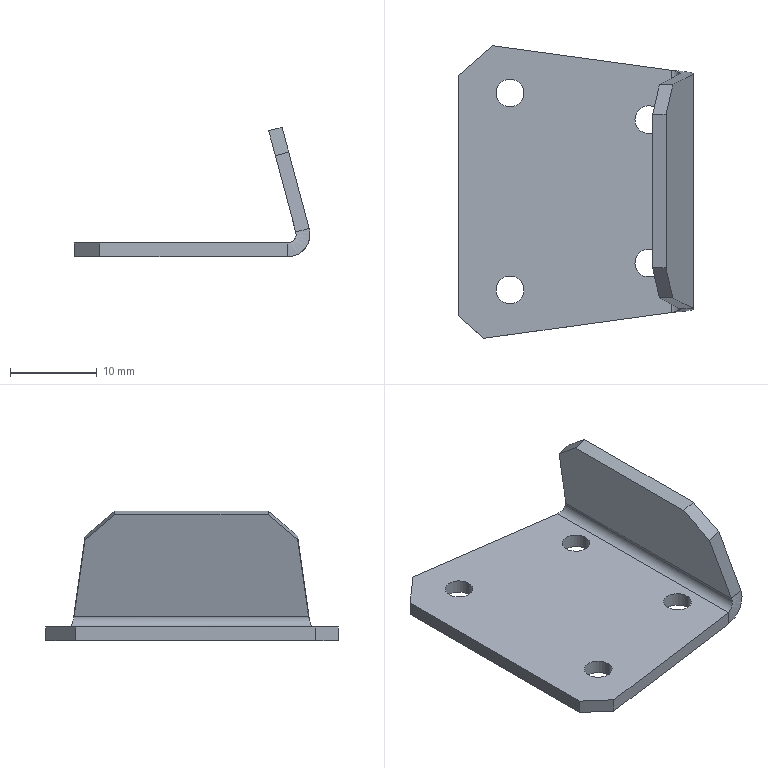Part | SolidWorks | features BaseBody 1 | 1 solid | 26 faces | box 27.212 x 33.746 x 14.951 mm | volume 1783 mm3 | plane 14 | cylinder 10 | spline 2 | commonest cylinder face diameters 3.2 x8 2 x1 5.2 x1
STEP:
#1=CARTESIAN_POINT('',(3.6,8.269,-1.6));
#2=VERTEX_POINT('',#1);
#3=CARTESIAN_POINT('',(0.4,8.269,-1.6));
#4=VERTEX_POINT('',#3);
#5=CARTESIAN_POINT('',(2.,8.269,-1.6));
#6=DIRECTION('',(0.,0.,-1.));
#7=DIRECTION('',(1.,0.,0.));
#8=AXIS2_PLACEMENT_3D('',#5,#6,#7);
#9=CIRCLE('',#8,1.6);
#10=EDGE_CURVE('',#2,#4,#9,.T.);
#11=ORIENTED_EDGE('',*,*,#10,.T.);
#12=CARTESIAN_POINT('',(0.4,8.269,0.));
#13=VERTEX_POINT('',#12);
#14=CARTESIAN_POINT('',(0.4,8.269,-1.6));
#15=DIRECTION('',(0.,0.,1.));
#16=VECTOR('',#15,1000.);
#17=LINE('',#14,#16);
#18=EDGE_CURVE('',#4,#13,#17,.T.);
#19=ORIENTED_EDGE('',*,*,#18,.T.);
#20=CARTESIAN_POINT('',(3.6,8.269,0.));
#21=VERTEX_POINT('',#20);
#22=CARTESIAN_POINT('',(2.,8.269,0.));
#23=DIRECTION('',(0.,0.,-1.));
#24=DIRECTION('',(1.,0.,0.));
#25=AXIS2_PLACEMENT_3D('',#22,#23,#24);
#26=CIRCLE('',#25,1.6);
#27=EDGE_CURVE('',#21,#13,#26,.T.);
#28=ORIENTED_EDGE('',*,*,#27,.F.);
#29=CARTESIAN_POINT('',(3.6,8.269,-1.6));
#30=DIRECTION('',(0.,0.,1.));
#31=VECTOR('',#30,1000.);
#32=LINE('',#29,#31);
#33=EDGE_CURVE('',#2,#21,#32,.T.);
#34=ORIENTED_EDGE('',*,*,#33,.F.);
#35=EDGE_LOOP('',(#11,#19,#28,#34));
#36=FACE_OUTER_BOUND('',#35,.T.);
#37=CARTESIAN_POINT('',(2.,8.269,-1.6));
#38=DIRECTION('',(0.,0.,1.));
#39=DIRECTION('',(1.,0.,0.));
#40=AXIS2_PLACEMENT_3D('',#37,#38,#39);
#41=CYLINDRICAL_SURFACE('',#40,1.6);
#42=ADVANCED_FACE('',(#36),#41,.F.);
#43=CARTESIAN_POINT('',(3.6,-8.269,-1.6));
#44=VERTEX_POINT('',#43);
#45=CARTESIAN_POINT('',(0.4,-8.269,-1.6));
#46=VERTEX_POINT('',#45);
#47=CARTESIAN_POINT('',(2.,-8.269,-1.6));
#48=DIRECTION('',(0.,0.,-1.));
#49=DIRECTION('',(1.,0.,0.));
#50=AXIS2_PLACEMENT_3D('',#47,#48,#49);
#51=CIRCLE('',#50,1.6);
#52=EDGE_CURVE('',#44,#46,#51,.T.);
#53=ORIENTED_EDGE('',*,*,#52,.T.);
#54=CARTESIAN_POINT('',(0.4,-8.269,0.));
#55=VERTEX_POINT('',#54);
#56=CARTESIAN_POINT('',(0.4,-8.269,-1.6));
#57=DIRECTION('',(0.,0.,1.));
#58=VECTOR('',#57,1000.);
#59=LINE('',#56,#58);
#60=EDGE_CURVE('',#46,#55,#59,.T.);
#61=ORIENTED_EDGE('',*,*,#60,.T.);
#62=CARTESIAN_POINT('',(3.6,-8.269,0.));
#63=VERTEX_POINT('',#62);
#64=CARTESIAN_POINT('',(2.,-8.269,0.));
#65=DIRECTION('',(0.,0.,-1.));
#66=DIRECTION('',(1.,0.,0.));
#67=AXIS2_PLACEMENT_3D('',#64,#65,#66);
#68=CIRCLE('',#67,1.6);
#69=EDGE_CURVE('',#63,#55,#68,.T.);
#70=ORIENTED_EDGE('',*,*,#69,.F.);
#71=CARTESIAN_POINT('',(3.6,-8.269,-1.6));
#72=DIRECTION('',(0.,0.,1.));
#73=VECTOR('',#72,1000.);
#74=LINE('',#71,#73);
#75=EDGE_CURVE('',#44,#63,#74,.T.);
#76=ORIENTED_EDGE('',*,*,#75,.F.);
#77=EDGE_LOOP('',(#53,#61,#70,#76));
#78=FACE_OUTER_BOUND('',#77,.T.);
#79=CARTESIAN_POINT('',(2.,-8.269,-1.6));
#80=DIRECTION('',(0.,0.,1.));
#81=DIRECTION('',(1.,0.,0.));
#82=AXIS2_PLACEMENT_3D('',#79,#80,#81);
#83=CYLINDRICAL_SURFACE('',#82,1.6);
#84=ADVANCED_FACE('',(#78),#83,.F.);
#85=CARTESIAN_POINT('',(-12.4,-11.35,-1.6));
#86=VERTEX_POINT('',#85);
#87=CARTESIAN_POINT('',(-15.6,-11.35,-1.6));
#88=VERTEX_POINT('',#87);
#89=CARTESIAN_POINT('',(-14.,-11.35,-1.6));
#90=DIRECTION('',(0.,0.,-1.));
#91=DIRECTION('',(1.,0.,0.));
#92=AXIS2_PLACEMENT_3D('',#89,#90,#91);
#93=CIRCLE('',#92,1.6);
#94=EDGE_CURVE('',#86,#88,#93,.T.);
#95=ORIENTED_EDGE('',*,*,#94,.T.);
#96=CARTESIAN_POINT('',(-15.6,-11.35,0.));
#97=VERTEX_POINT('',#96);
#98=CARTESIAN_POINT('',(-15.6,-11.35,-1.6));
#99=DIRECTION('',(0.,0.,1.));
#100=VECTOR('',#99,1000.);
#101=LINE('',#98,#100);
#102=EDGE_CURVE('',#88,#97,#101,.T.);
#103=ORIENTED_EDGE('',*,*,#102,.T.);
#104=CARTESIAN_POINT('',(-12.4,-11.35,0.));
#105=VERTEX_POINT('',#104);
#106=CARTESIAN_POINT('',(-14.,-11.35,0.));
#107=DIRECTION('',(0.,0.,-1.));
#108=DIRECTION('',(1.,0.,0.));
#109=AXIS2_PLACEMENT_3D('',#106,#107,#108);
#110=CIRCLE('',#109,1.6);
#111=EDGE_CURVE('',#105,#97,#110,.T.);
#112=ORIENTED_EDGE('',*,*,#111,.F.);
#113=CARTESIAN_POINT('',(-12.4,-11.35,-1.6));
#114=DIRECTION('',(0.,0.,1.));
#115=VECTOR('',#114,1000.);
#116=LINE('',#113,#115);
#117=EDGE_CURVE('',#86,#105,#116,.T.);
#118=ORIENTED_EDGE('',*,*,#117,.F.);
#119=EDGE_LOOP('',(#95,#103,#112,#118));
#120=FACE_OUTER_BOUND('',#119,.T.);
#121=CARTESIAN_POINT('',(-14.,-11.35,-1.6));
#122=DIRECTION('',(0.,0.,1.));
#123=DIRECTION('',(1.,0.,0.));
#124=AXIS2_PLACEMENT_3D('',#121,#122,#123);
#125=CYLINDRICAL_SURFACE('',#124,1.6);
#126=ADVANCED_FACE('',(#120),#125,.F.);
#127=CARTESIAN_POINT('',(-12.4,11.35,-1.6));
#128=VERTEX_POINT('',#127);
#129=CARTESIAN_POINT('',(-15.6,11.35,-1.6));
#130=VERTEX_POINT('',#129);
#131=CARTESIAN_POINT('',(-14.,11.35,-1.6));
#132=DIRECTION('',(0.,0.,-1.));
#133=DIRECTION('',(1.,0.,0.));
#134=AXIS2_PLACEMENT_3D('',#131,#132,#133);
#135=CIRCLE('',#134,1.6);
#136=EDGE_CURVE('',#128,#130,#135,.T.);
#137=ORIENTED_EDGE('',*,*,#136,.T.);
#138=CARTESIAN_POINT('',(-15.6,11.35,0.));
#139=VERTEX_POINT('',#138);
#140=CARTESIAN_POINT('',(-15.6,11.35,-1.6));
#141=DIRECTION('',(0.,0.,1.));
#142=VECTOR('',#141,1000.);
#143=LINE('',#140,#142);
#144=EDGE_CURVE('',#130,#139,#143,.T.);
#145=ORIENTED_EDGE('',*,*,#144,.T.);
#146=CARTESIAN_POINT('',(-12.4,11.35,0.));
#147=VERTEX_POINT('',#146);
#148=CARTESIAN_POINT('',(-14.,11.35,0.));
#149=DIRECTION('',(0.,0.,-1.));
#150=DIRECTION('',(1.,0.,0.));
#151=AXIS2_PLACEMENT_3D('',#148,#149,#150);
#152=CIRCLE('',#151,1.6);
#153=EDGE_CURVE('',#147,#139,#152,.T.);
#154=ORIENTED_EDGE('',*,*,#153,.F.);
#155=CARTESIAN_POINT('',(-12.4,11.35,-1.6));
#156=DIRECTION('',(0.,0.,1.));
#157=VECTOR('',#156,1000.);
#158=LINE('',#155,#157);
#159=EDGE_CURVE('',#128,#147,#158,.T.);
#160=ORIENTED_EDGE('',*,*,#159,.F.);
#161=EDGE_LOOP('',(#137,#145,#154,#160));
#162=FACE_OUTER_BOUND('',#161,.T.);
#163=CARTESIAN_POINT('',(-14.,11.35,-1.6));
#164=DIRECTION('',(0.,0.,1.));
#165=DIRECTION('',(1.,0.,0.));
#166=AXIS2_PLACEMENT_3D('',#163,#164,#165);
#167=CYLINDRICAL_SURFACE('',#166,1.6);
#168=ADVANCED_FACE('',(#162),#167,.F.);
#169=CARTESIAN_POINT('',(5.578,-13.512,1.259));
#170=VERTEX_POINT('',#169);
#171=CARTESIAN_POINT('',(4.612,-13.966,0.));
#172=VERTEX_POINT('',#171);
#173=CARTESIAN_POINT('',(5.578,-13.512,1.259));
#174=CARTESIAN_POINT('',(5.617,-13.55,1.11));
#175=CARTESIAN_POINT('',(5.622,-13.588,0.9534));
#176=CARTESIAN_POINT('',(5.563,-13.663,0.6556));
#177=CARTESIAN_POINT('',(5.498,-13.701,0.513));
#178=CARTESIAN_POINT('',(5.312,-13.777,0.2701));
#179=CARTESIAN_POINT('',(5.191,-13.815,0.1708));
#180=CARTESIAN_POINT('',(4.917,-13.89,0.03575));
#181=CARTESIAN_POINT('',(4.766,-13.928,0.));
#182=CARTESIAN_POINT('',(4.612,-13.966,0.));
#183=B_SPLINE_CURVE_WITH_KNOTS('',3,(#173,#174,#175,#176,#177,#178,#179,#180,#181,#182),.UNSPECIFIED.,.F.,.F.,(4,2,2,2,4),(-0.0002673,0.0002018,0.000671,0.00114,0.001609),.UNSPECIFIED.);
#184=EDGE_CURVE('',#170,#172,#183,.T.);
#185=ORIENTED_EDGE('',*,*,#184,.F.);
#186=CARTESIAN_POINT('',(5.578,13.512,1.259));
#187=VERTEX_POINT('',#186);
#188=CARTESIAN_POINT('',(5.578,0.,1.259));
#189=DIRECTION('',(0.,1.,0.));
#190=VECTOR('',#189,1000.);
#191=LINE('',#188,#190);
#192=EDGE_CURVE('',#170,#187,#191,.T.);
#193=ORIENTED_EDGE('',*,*,#192,.T.);
#194=CARTESIAN_POINT('',(4.612,13.966,0.));
#195=VERTEX_POINT('',#194);
#196=CARTESIAN_POINT('',(4.612,13.966,0.));
#197=CARTESIAN_POINT('',(4.689,13.947,0.));
#198=CARTESIAN_POINT('',(4.764,13.928,0.008783));
#199=CARTESIAN_POINT('',(4.912,13.891,0.04322));
#200=CARTESIAN_POINT('',(4.985,13.871,0.06937));
#201=CARTESIAN_POINT('',(5.19,13.815,0.1702));
#202=CARTESIAN_POINT('',(5.311,13.777,0.2697));
#203=CARTESIAN_POINT('',(5.45,13.721,0.4504));
#204=CARTESIAN_POINT('',(5.491,13.702,0.517));
#205=CARTESIAN_POINT('',(5.553,13.664,0.6555));
#206=CARTESIAN_POINT('',(5.577,13.645,0.7278));
#207=CARTESIAN_POINT('',(5.622,13.588,0.9536));
#208=CARTESIAN_POINT('',(5.617,13.55,1.11));
#209=CARTESIAN_POINT('',(5.578,13.512,1.259));
#210=B_SPLINE_CURVE_WITH_KNOTS('',3,(#196,#197,#198,#199,#200,#201,#202,#203,#204,#205,#206,#207,#208,#209),.UNSPECIFIED.,.F.,.F.,(4,2,2,2,2,2,4),(-0.001619,-0.001383,-0.001147,-0.0006751,-0.0004391,-0.0002031,0.000269),.UNSPECIFIED.);
#211=EDGE_CURVE('',#195,#187,#210,.T.);
#212=ORIENTED_EDGE('',*,*,#211,.F.);
#213=CARTESIAN_POINT('',(4.612,0.,0.));
#214=DIRECTION('',(0.,-1.,0.));
#215=VECTOR('',#214,1000.);
#216=LINE('',#213,#215);
#217=EDGE_CURVE('',#195,#172,#216,.T.);
#218=ORIENTED_EDGE('',*,*,#217,.T.);
#219=EDGE_LOOP('',(#185,#193,#212,#218));
#220=FACE_OUTER_BOUND('',#219,.T.);
#221=CARTESIAN_POINT('',(4.612,13.74,1.));
#222=DIRECTION('',(0.,-1.,0.));
#223=DIRECTION('',(0.,0.,-1.));
#224=AXIS2_PLACEMENT_3D('',#221,#222,#223);
#225=CYLINDRICAL_SURFACE('',#224,1.);
#226=ADVANCED_FACE('',(#220),#225,.F.);
#227=CARTESIAN_POINT('',(2.448,8.85,12.937));
#228=VERTEX_POINT('',#227);
#229=CARTESIAN_POINT('',(3.218,12.259,10.066));
#230=VERTEX_POINT('',#229);
#231=CARTESIAN_POINT('',(2.448,8.85,12.937));
#232=DIRECTION('',(0.1701,0.7537,-0.6348));
#233=VECTOR('',#232,1000.);
#234=LINE('',#231,#233);
#235=EDGE_CURVE('',#228,#230,#234,.T.);
#236=ORIENTED_EDGE('',*,*,#235,.T.);
#237=CARTESIAN_POINT('',(3.218,12.259,10.066));
#238=DIRECTION('',(0.2564,0.1362,-0.9569));
#239=VECTOR('',#238,1000.);
#240=LINE('',#237,#239);
#241=EDGE_CURVE('',#230,#187,#240,.T.);
#242=ORIENTED_EDGE('',*,*,#241,.T.);
#243=ORIENTED_EDGE('',*,*,#192,.F.);
#244=CARTESIAN_POINT('',(3.218,-12.259,10.066));
#245=VERTEX_POINT('',#244);
#246=CARTESIAN_POINT('',(5.578,-13.512,1.259));
#247=DIRECTION('',(-0.2564,0.1362,0.9569));
#248=VECTOR('',#247,1000.);
#249=LINE('',#246,#248);
#250=EDGE_CURVE('',#170,#245,#249,.T.);
#251=ORIENTED_EDGE('',*,*,#250,.T.);
#252=CARTESIAN_POINT('',(2.448,-8.85,12.937));
#253=VERTEX_POINT('',#252);
#254=CARTESIAN_POINT('',(3.218,-12.259,10.066));
#255=DIRECTION('',(-0.1701,0.7537,0.6348));
#256=VECTOR('',#255,1000.);
#257=LINE('',#254,#256);
#258=EDGE_CURVE('',#245,#253,#257,.T.);
#259=ORIENTED_EDGE('',*,*,#258,.T.);
#260=CARTESIAN_POINT('',(2.448,0.,12.937));
#261=DIRECTION('',(0.,1.,0.));
#262=VECTOR('',#261,1000.);
#263=LINE('',#260,#262);
#264=EDGE_CURVE('',#253,#228,#263,.T.);
#265=ORIENTED_EDGE('',*,*,#264,.T.);
#266=EDGE_LOOP('',(#236,#242,#243,#251,#259,#265));
#267=FACE_OUTER_BOUND('',#266,.T.);
#268=CARTESIAN_POINT('',(5.578,-13.512,1.259));
#269=DIRECTION('',(-0.9659,0.,-0.2588));
#270=DIRECTION('',(-0.2588,0.,0.9659));
#271=AXIS2_PLACEMENT_3D('',#268,#269,#270);
#272=PLANE('',#271);
#273=ADVANCED_FACE('',(#267),#272,.T.);
#274=CARTESIAN_POINT('',(4.763,12.259,10.48));
#275=VERTEX_POINT('',#274);
#276=CARTESIAN_POINT('',(3.99,12.259,10.273));
#277=DIRECTION('',(0.9659,0.,0.2588));
#278=VECTOR('',#277,1000.);
#279=LINE('',#276,#278);
#280=EDGE_CURVE('',#230,#275,#279,.T.);
#281=ORIENTED_EDGE('',*,*,#280,.T.);
#282=CARTESIAN_POINT('',(7.123,13.512,1.673));
#283=VERTEX_POINT('',#282);
#284=CARTESIAN_POINT('',(5.943,12.885,6.076));
#285=DIRECTION('',(0.2564,0.1362,-0.9569));
#286=VECTOR('',#285,1000.);
#287=LINE('',#284,#286);
#288=EDGE_CURVE('',#275,#283,#287,.T.);
#289=ORIENTED_EDGE('',*,*,#288,.T.);
#290=CARTESIAN_POINT('',(6.35,13.512,1.466));
#291=DIRECTION('',(0.9659,0.,0.2588));
#292=VECTOR('',#291,1000.);
#293=LINE('',#290,#292);
#294=EDGE_CURVE('',#187,#283,#293,.T.);
#295=ORIENTED_EDGE('',*,*,#294,.F.);
#296=ORIENTED_EDGE('',*,*,#241,.F.);
#297=EDGE_LOOP('',(#281,#289,#295,#296));
#298=FACE_OUTER_BOUND('',#297,.T.);
#299=CARTESIAN_POINT('',(4.763,12.259,10.48));
#300=DIRECTION('',(-0.03526,0.9907,0.1316));
#301=DIRECTION('',(0.2564,0.1362,-0.9569));
#302=AXIS2_PLACEMENT_3D('',#299,#300,#301);
#303=PLANE('',#302);
#304=ADVANCED_FACE('',(#298),#303,.T.);
#305=CARTESIAN_POINT('',(3.994,8.85,13.351));
#306=VERTEX_POINT('',#305);
#307=CARTESIAN_POINT('',(4.379,10.554,11.915));
#308=DIRECTION('',(0.1701,0.7537,-0.6348));
#309=VECTOR('',#308,1000.);
#310=LINE('',#307,#309);
#311=EDGE_CURVE('',#306,#275,#310,.T.);
#312=ORIENTED_EDGE('',*,*,#311,.T.);
#313=ORIENTED_EDGE('',*,*,#280,.F.);
#314=ORIENTED_EDGE('',*,*,#235,.F.);
#315=CARTESIAN_POINT('',(3.221,8.85,13.144));
#316=DIRECTION('',(0.9659,0.,0.2588));
#317=VECTOR('',#316,1000.);
#318=LINE('',#315,#317);
#319=EDGE_CURVE('',#228,#306,#318,.T.);
#320=ORIENTED_EDGE('',*,*,#319,.T.);
#321=EDGE_LOOP('',(#312,#313,#314,#320));
#322=FACE_OUTER_BOUND('',#321,.T.);
#323=CARTESIAN_POINT('',(3.994,8.85,13.351));
#324=DIRECTION('',(-0.1951,0.6572,0.728));
#325=DIRECTION('',(0.1701,0.7537,-0.6348));
#326=AXIS2_PLACEMENT_3D('',#323,#324,#325);
#327=PLANE('',#326);
#328=ADVANCED_FACE('',(#322),#327,.T.);
#329=CARTESIAN_POINT('',(3.994,-8.85,13.351));
#330=VERTEX_POINT('',#329);
#331=CARTESIAN_POINT('',(3.994,0.,13.351));
#332=DIRECTION('',(0.,1.,0.));
#333=VECTOR('',#332,1000.);
#334=LINE('',#331,#333);
#335=EDGE_CURVE('',#330,#306,#334,.T.);
#336=ORIENTED_EDGE('',*,*,#335,.T.);
#337=ORIENTED_EDGE('',*,*,#319,.F.);
#338=ORIENTED_EDGE('',*,*,#264,.F.);
#339=CARTESIAN_POINT('',(3.221,-8.85,13.144));
#340=DIRECTION('',(0.9659,0.,0.2588));
#341=VECTOR('',#340,1000.);
#342=LINE('',#339,#341);
#343=EDGE_CURVE('',#253,#330,#342,.T.);
#344=ORIENTED_EDGE('',*,*,#343,.T.);
#345=EDGE_LOOP('',(#336,#337,#338,#344));
#346=FACE_OUTER_BOUND('',#345,.T.);
#347=CARTESIAN_POINT('',(2.448,-8.85,12.937));
#348=DIRECTION('',(-0.2588,0.,0.9659));
#349=DIRECTION('',(0.9659,0.,0.2588));
#350=AXIS2_PLACEMENT_3D('',#347,#348,#349);
#351=PLANE('',#350);
#352=ADVANCED_FACE('',(#346),#351,.T.);
#353=CARTESIAN_POINT('',(4.763,-12.259,10.48));
#354=VERTEX_POINT('',#353);
#355=CARTESIAN_POINT('',(4.379,-10.554,11.915));
#356=DIRECTION('',(-0.1701,0.7537,0.6348));
#357=VECTOR('',#356,1000.);
#358=LINE('',#355,#357);
#359=EDGE_CURVE('',#354,#330,#358,.T.);
#360=ORIENTED_EDGE('',*,*,#359,.T.);
#361=ORIENTED_EDGE('',*,*,#343,.F.);
#362=ORIENTED_EDGE('',*,*,#258,.F.);
#363=CARTESIAN_POINT('',(3.99,-12.259,10.273));
#364=DIRECTION('',(0.9659,0.,0.2588));
#365=VECTOR('',#364,1000.);
#366=LINE('',#363,#365);
#367=EDGE_CURVE('',#245,#354,#366,.T.);
#368=ORIENTED_EDGE('',*,*,#367,.T.);
#369=EDGE_LOOP('',(#360,#361,#362,#368));
#370=FACE_OUTER_BOUND('',#369,.T.);
#371=CARTESIAN_POINT('',(4.763,-12.259,10.48));
#372=DIRECTION('',(-0.1951,-0.6572,0.728));
#373=DIRECTION('',(-0.1701,0.7537,0.6348));
#374=AXIS2_PLACEMENT_3D('',#371,#372,#373);
#375=PLANE('',#374);
#376=ADVANCED_FACE('',(#370),#375,.T.);
#377=ORIENTED_EDGE('',*,*,#367,.F.);
#378=ORIENTED_EDGE('',*,*,#250,.F.);
#379=CARTESIAN_POINT('',(7.123,-13.512,1.673));
#380=VERTEX_POINT('',#379);
#381=CARTESIAN_POINT('',(6.35,-13.512,1.466));
#382=DIRECTION('',(-0.9659,0.,-0.2588));
#383=VECTOR('',#382,1000.);
#384=LINE('',#381,#383);
#385=EDGE_CURVE('',#380,#170,#384,.T.);
#386=ORIENTED_EDGE('',*,*,#385,.F.);
#387=CARTESIAN_POINT('',(5.943,-12.885,6.076));
#388=DIRECTION('',(-0.2564,0.1362,0.9569));
#389=VECTOR('',#388,1000.);
#390=LINE('',#387,#389);
#391=EDGE_CURVE('',#380,#354,#390,.T.);
#392=ORIENTED_EDGE('',*,*,#391,.T.);
#393=EDGE_LOOP('',(#377,#378,#386,#392));
#394=FACE_OUTER_BOUND('',#393,.T.);
#395=CARTESIAN_POINT('',(7.123,-13.512,1.673));
#396=DIRECTION('',(-0.03526,-0.9907,0.1316));
#397=DIRECTION('',(-0.2564,0.1362,0.9569));
#398=AXIS2_PLACEMENT_3D('',#395,#396,#397);
#399=PLANE('',#398);
#400=ADVANCED_FACE('',(#394),#399,.T.);
#401=ORIENTED_EDGE('',*,*,#27,.T.);
#402=CARTESIAN_POINT('',(2.,8.269,0.));
#403=DIRECTION('',(0.,0.,-1.));
#404=DIRECTION('',(1.,0.,0.));
#405=AXIS2_PLACEMENT_3D('',#402,#403,#404);
#406=CIRCLE('',#405,1.6);
#407=EDGE_CURVE('',#13,#21,#406,.T.);
#408=ORIENTED_EDGE('',*,*,#407,.T.);
#409=EDGE_LOOP('',(#401,#408));
#410=FACE_BOUND('',#409,.T.);
#411=ORIENTED_EDGE('',*,*,#69,.T.);
#412=CARTESIAN_POINT('',(2.,-8.269,0.));
#413=DIRECTION('',(0.,0.,-1.));
#414=DIRECTION('',(1.,0.,0.));
#415=AXIS2_PLACEMENT_3D('',#412,#413,#414);
#416=CIRCLE('',#415,1.6);
#417=EDGE_CURVE('',#55,#63,#416,.T.);
#418=ORIENTED_EDGE('',*,*,#417,.T.);
#419=EDGE_LOOP('',(#411,#418));
#420=FACE_BOUND('',#419,.T.);
#421=ORIENTED_EDGE('',*,*,#111,.T.);
#422=CARTESIAN_POINT('',(-14.,-11.35,0.));
#423=DIRECTION('',(0.,0.,-1.));
#424=DIRECTION('',(1.,0.,0.));
#425=AXIS2_PLACEMENT_3D('',#422,#423,#424);
#426=CIRCLE('',#425,1.6);
#427=EDGE_CURVE('',#97,#105,#426,.T.);
#428=ORIENTED_EDGE('',*,*,#427,.T.);
#429=EDGE_LOOP('',(#421,#428));
#430=FACE_BOUND('',#429,.T.);
#431=ORIENTED_EDGE('',*,*,#153,.T.);
#432=CARTESIAN_POINT('',(-14.,11.35,0.));
#433=DIRECTION('',(0.,0.,-1.));
#434=DIRECTION('',(1.,0.,0.));
#435=AXIS2_PLACEMENT_3D('',#432,#433,#434);
#436=CIRCLE('',#435,1.6);
#437=EDGE_CURVE('',#139,#147,#436,.T.);
#438=ORIENTED_EDGE('',*,*,#437,.T.);
#439=EDGE_LOOP('',(#431,#438));
#440=FACE_BOUND('',#439,.T.);
#441=CARTESIAN_POINT('',(-20.,13.35,0.));
#442=VERTEX_POINT('',#441);
#443=CARTESIAN_POINT('',(-20.,-14.35,0.));
#444=VERTEX_POINT('',#443);
#445=CARTESIAN_POINT('',(-20.,-0.06811,0.));
#446=DIRECTION('',(0.,-1.,0.));
#447=VECTOR('',#446,1000.);
#448=LINE('',#445,#447);
#449=EDGE_CURVE('',#442,#444,#448,.T.);
#450=ORIENTED_EDGE('',*,*,#449,.T.);
#451=CARTESIAN_POINT('',(-17.028,-16.941,0.));
#452=VERTEX_POINT('',#451);
#453=CARTESIAN_POINT('',(-20.,-14.35,0.));
#454=DIRECTION('',(0.7537,-0.6572,0.));
#455=VECTOR('',#454,1000.);
#456=LINE('',#453,#455);
#457=EDGE_CURVE('',#444,#452,#456,.T.);
#458=ORIENTED_EDGE('',*,*,#457,.T.);
#459=CARTESIAN_POINT('',(-17.028,-16.941,0.));
#460=DIRECTION('',(0.9907,0.1362,0.));
#461=VECTOR('',#460,1000.);
#462=LINE('',#459,#461);
#463=EDGE_CURVE('',#452,#172,#462,.T.);
#464=ORIENTED_EDGE('',*,*,#463,.T.);
#465=ORIENTED_EDGE('',*,*,#217,.F.);
#466=CARTESIAN_POINT('',(-16.037,16.805,0.));
#467=VERTEX_POINT('',#466);
#468=CARTESIAN_POINT('',(4.612,13.966,0.));
#469=DIRECTION('',(-0.9907,0.1362,0.));
#470=VECTOR('',#469,1000.);
#471=LINE('',#468,#470);
#472=EDGE_CURVE('',#195,#467,#471,.T.);
#473=ORIENTED_EDGE('',*,*,#472,.T.);
#474=CARTESIAN_POINT('',(-16.037,16.805,0.));
#475=DIRECTION('',(-0.7537,-0.6572,0.));
#476=VECTOR('',#475,1000.);
#477=LINE('',#474,#476);
#478=EDGE_CURVE('',#467,#442,#477,.T.);
#479=ORIENTED_EDGE('',*,*,#478,.T.);
#480=EDGE_LOOP('',(#450,#458,#464,#465,#473,#479));
#481=FACE_OUTER_BOUND('',#480,.T.);
#482=CARTESIAN_POINT('',(-20.,-17.144,0.));
#483=DIRECTION('',(0.,0.,1.));
#484=DIRECTION('',(1.,0.,0.));
#485=AXIS2_PLACEMENT_3D('',#482,#483,#484);
#486=PLANE('',#485);
#487=ADVANCED_FACE('',(#410,#420,#430,#440,#481),#486,.T.);
#488=CARTESIAN_POINT('',(7.123,0.,1.673));
#489=DIRECTION('',(0.,-1.,0.));
#490=VECTOR('',#489,1000.);
#491=LINE('',#488,#490);
#492=EDGE_CURVE('',#283,#380,#491,.T.);
#493=ORIENTED_EDGE('',*,*,#492,.F.);
#494=ORIENTED_EDGE('',*,*,#288,.F.);
#495=ORIENTED_EDGE('',*,*,#311,.F.);
#496=ORIENTED_EDGE('',*,*,#335,.F.);
#497=ORIENTED_EDGE('',*,*,#359,.F.);
#498=ORIENTED_EDGE('',*,*,#391,.F.);
#499=EDGE_LOOP('',(#493,#494,#495,#496,#497,#498));
#500=FACE_OUTER_BOUND('',#499,.T.);
#501=CARTESIAN_POINT('',(7.123,-13.512,1.673));
#502=DIRECTION('',(-0.9659,0.,-0.2588));
#503=DIRECTION('',(-0.2588,0.,0.9659));
#504=AXIS2_PLACEMENT_3D('',#501,#502,#503);
#505=PLANE('',#504);
#506=ADVANCED_FACE('',(#500),#505,.F.);
#507=ORIENTED_EDGE('',*,*,#18,.F.);
#508=CARTESIAN_POINT('',(2.,8.269,-1.6));
#509=DIRECTION('',(0.,0.,-1.));
#510=DIRECTION('',(1.,0.,0.));
#511=AXIS2_PLACEMENT_3D('',#508,#509,#510);
#512=CIRCLE('',#511,1.6);
#513=EDGE_CURVE('',#4,#2,#512,.T.);
#514=ORIENTED_EDGE('',*,*,#513,.T.);
#515=ORIENTED_EDGE('',*,*,#33,.T.);
#516=ORIENTED_EDGE('',*,*,#407,.F.);
#517=EDGE_LOOP('',(#507,#514,#515,#516));
#518=FACE_OUTER_BOUND('',#517,.T.);
#519=CARTESIAN_POINT('',(2.,8.269,-1.6));
#520=DIRECTION('',(0.,0.,1.));
#521=DIRECTION('',(1.,0.,0.));
#522=AXIS2_PLACEMENT_3D('',#519,#520,#521);
#523=CYLINDRICAL_SURFACE('',#522,1.6);
#524=ADVANCED_FACE('',(#518),#523,.F.);
#525=ORIENTED_EDGE('',*,*,#60,.F.);
#526=CARTESIAN_POINT('',(2.,-8.269,-1.6));
#527=DIRECTION('',(0.,0.,-1.));
#528=DIRECTION('',(1.,0.,0.));
#529=AXIS2_PLACEMENT_3D('',#526,#527,#528);
#530=CIRCLE('',#529,1.6);
#531=EDGE_CURVE('',#46,#44,#530,.T.);
#532=ORIENTED_EDGE('',*,*,#531,.T.);
#533=ORIENTED_EDGE('',*,*,#75,.T.);
#534=ORIENTED_EDGE('',*,*,#417,.F.);
#535=EDGE_LOOP('',(#525,#532,#533,#534));
#536=FACE_OUTER_BOUND('',#535,.T.);
#537=CARTESIAN_POINT('',(2.,-8.269,-1.6));
#538=DIRECTION('',(0.,0.,1.));
#539=DIRECTION('',(1.,0.,0.));
#540=AXIS2_PLACEMENT_3D('',#537,#538,#539);
#541=CYLINDRICAL_SURFACE('',#540,1.6);
#542=ADVANCED_FACE('',(#536),#541,.F.);
#543=ORIENTED_EDGE('',*,*,#102,.F.);
#544=CARTESIAN_POINT('',(-14.,-11.35,-1.6));
#545=DIRECTION('',(0.,0.,-1.));
#546=DIRECTION('',(1.,0.,0.));
#547=AXIS2_PLACEMENT_3D('',#544,#545,#546);
#548=CIRCLE('',#547,1.6);
#549=EDGE_CURVE('',#88,#86,#548,.T.);
#550=ORIENTED_EDGE('',*,*,#549,.T.);
#551=ORIENTED_EDGE('',*,*,#117,.T.);
#552=ORIENTED_EDGE('',*,*,#427,.F.);
#553=EDGE_LOOP('',(#543,#550,#551,#552));
#554=FACE_OUTER_BOUND('',#553,.T.);
#555=CARTESIAN_POINT('',(-14.,-11.35,-1.6));
#556=DIRECTION('',(0.,0.,1.));
#557=DIRECTION('',(1.,0.,0.));
#558=AXIS2_PLACEMENT_3D('',#555,#556,#557);
#559=CYLINDRICAL_SURFACE('',#558,1.6);
#560=ADVANCED_FACE('',(#554),#559,.F.);
#561=ORIENTED_EDGE('',*,*,#144,.F.);
#562=CARTESIAN_POINT('',(-14.,11.35,-1.6));
#563=DIRECTION('',(0.,0.,-1.));
#564=DIRECTION('',(1.,0.,0.));
#565=AXIS2_PLACEMENT_3D('',#562,#563,#564);
#566=CIRCLE('',#565,1.6);
#567=EDGE_CURVE('',#130,#128,#566,.T.);
#568=ORIENTED_EDGE('',*,*,#567,.T.);
#569=ORIENTED_EDGE('',*,*,#159,.T.);
#570=ORIENTED_EDGE('',*,*,#437,.F.);
#571=EDGE_LOOP('',(#561,#568,#569,#570));
#572=FACE_OUTER_BOUND('',#571,.T.);
#573=CARTESIAN_POINT('',(-14.,11.35,-1.6));
#574=DIRECTION('',(0.,0.,1.));
#575=DIRECTION('',(1.,0.,0.));
#576=AXIS2_PLACEMENT_3D('',#573,#574,#575);
#577=CYLINDRICAL_SURFACE('',#576,1.6);
#578=ADVANCED_FACE('',(#572),#577,.F.);
#579=CARTESIAN_POINT('',(-20.,-14.35,-1.6));
#580=VERTEX_POINT('',#579);
#581=CARTESIAN_POINT('',(-17.028,-16.941,-1.6));
#582=VERTEX_POINT('',#581);
#583=CARTESIAN_POINT('',(-18.514,-15.646,-1.6));
#584=DIRECTION('',(0.7537,-0.6572,0.));
#585=VECTOR('',#584,1000.);
#586=LINE('',#583,#585);
#587=EDGE_CURVE('',#580,#582,#586,.T.);
#588=ORIENTED_EDGE('',*,*,#587,.T.);
#589=CARTESIAN_POINT('',(-17.028,-16.941,-0.8));
#590=DIRECTION('',(0.,0.,1.));
#591=VECTOR('',#590,1000.);
#592=LINE('',#589,#591);
#593=EDGE_CURVE('',#582,#452,#592,.T.);
#594=ORIENTED_EDGE('',*,*,#593,.T.);
#595=ORIENTED_EDGE('',*,*,#457,.F.);
#596=CARTESIAN_POINT('',(-20.,-14.35,-0.8));
#597=DIRECTION('',(0.,0.,-1.));
#598=VECTOR('',#597,1000.);
#599=LINE('',#596,#598);
#600=EDGE_CURVE('',#444,#580,#599,.T.);
#601=ORIENTED_EDGE('',*,*,#600,.T.);
#602=EDGE_LOOP('',(#588,#594,#595,#601));
#603=FACE_OUTER_BOUND('',#602,.T.);
#604=CARTESIAN_POINT('',(-20.,-14.35,-1.6));
#605=DIRECTION('',(-0.6572,-0.7537,0.));
#606=DIRECTION('',(0.7537,-0.6572,0.));
#607=AXIS2_PLACEMENT_3D('',#604,#605,#606);
#608=PLANE('',#607);
#609=ADVANCED_FACE('',(#603),#608,.T.);
#610=CARTESIAN_POINT('',(-20.,13.35,-1.6));
#611=VERTEX_POINT('',#610);
#612=CARTESIAN_POINT('',(-20.,-0.5,-1.6));
#613=DIRECTION('',(0.,-1.,0.));
#614=VECTOR('',#613,1000.);
#615=LINE('',#612,#614);
#616=EDGE_CURVE('',#611,#580,#615,.T.);
#617=ORIENTED_EDGE('',*,*,#616,.T.);
#618=ORIENTED_EDGE('',*,*,#600,.F.);
#619=ORIENTED_EDGE('',*,*,#449,.F.);
#620=CARTESIAN_POINT('',(-20.,13.35,-0.8));
#621=DIRECTION('',(0.,0.,-1.));
#622=VECTOR('',#621,1000.);
#623=LINE('',#620,#622);
#624=EDGE_CURVE('',#442,#611,#623,.T.);
#625=ORIENTED_EDGE('',*,*,#624,.T.);
#626=EDGE_LOOP('',(#617,#618,#619,#625));
#627=FACE_OUTER_BOUND('',#626,.T.);
#628=CARTESIAN_POINT('',(-20.,13.35,-1.6));
#629=DIRECTION('',(-1.,0.,0.));
#630=DIRECTION('',(0.,-1.,0.));
#631=AXIS2_PLACEMENT_3D('',#628,#629,#630);
#632=PLANE('',#631);
#633=ADVANCED_FACE('',(#627),#632,.T.);
#634=CARTESIAN_POINT('',(-16.037,16.805,-1.6));
#635=VERTEX_POINT('',#634);
#636=CARTESIAN_POINT('',(-18.019,15.078,-1.6));
#637=DIRECTION('',(-0.7537,-0.6572,0.));
#638=VECTOR('',#637,1000.);
#639=LINE('',#636,#638);
#640=EDGE_CURVE('',#635,#611,#639,.T.);
#641=ORIENTED_EDGE('',*,*,#640,.T.);
#642=ORIENTED_EDGE('',*,*,#624,.F.);
#643=ORIENTED_EDGE('',*,*,#478,.F.);
#644=CARTESIAN_POINT('',(-16.037,16.805,-0.8));
#645=DIRECTION('',(0.,0.,-1.));
#646=VECTOR('',#645,1000.);
#647=LINE('',#644,#646);
#648=EDGE_CURVE('',#467,#635,#647,.T.);
#649=ORIENTED_EDGE('',*,*,#648,.T.);
#650=EDGE_LOOP('',(#641,#642,#643,#649));
#651=FACE_OUTER_BOUND('',#650,.T.);
#652=CARTESIAN_POINT('',(-16.037,16.805,-1.6));
#653=DIRECTION('',(-0.6572,0.7537,0.));
#654=DIRECTION('',(-0.7537,-0.6572,0.));
#655=AXIS2_PLACEMENT_3D('',#652,#653,#654);
#656=PLANE('',#655);
#657=ADVANCED_FACE('',(#651),#656,.T.);
#658=CARTESIAN_POINT('',(4.612,13.966,-1.6));
#659=VERTEX_POINT('',#658);
#660=CARTESIAN_POINT('',(-5.713,15.386,-1.6));
#661=DIRECTION('',(-0.9907,0.1362,0.));
#662=VECTOR('',#661,1000.);
#663=LINE('',#660,#662);
#664=EDGE_CURVE('',#659,#635,#663,.T.);
#665=ORIENTED_EDGE('',*,*,#664,.T.);
#666=ORIENTED_EDGE('',*,*,#648,.F.);
#667=ORIENTED_EDGE('',*,*,#472,.F.);
#668=CARTESIAN_POINT('',(4.612,13.966,-0.8));
#669=DIRECTION('',(0.,0.,1.));
#670=VECTOR('',#669,1000.);
#671=LINE('',#668,#670);
#672=EDGE_CURVE('',#659,#195,#671,.T.);
#673=ORIENTED_EDGE('',*,*,#672,.F.);
#674=EDGE_LOOP('',(#665,#666,#667,#673));
#675=FACE_OUTER_BOUND('',#674,.T.);
#676=CARTESIAN_POINT('',(4.612,13.966,-1.6));
#677=DIRECTION('',(0.1362,0.9907,0.));
#678=DIRECTION('',(-0.9907,0.1362,0.));
#679=AXIS2_PLACEMENT_3D('',#676,#677,#678);
#680=PLANE('',#679);
#681=ADVANCED_FACE('',(#675),#680,.T.);
#682=ORIENTED_EDGE('',*,*,#463,.F.);
#683=ORIENTED_EDGE('',*,*,#593,.F.);
#684=CARTESIAN_POINT('',(4.612,-13.966,-1.6));
#685=VERTEX_POINT('',#684);
#686=CARTESIAN_POINT('',(-6.208,-15.454,-1.6));
#687=DIRECTION('',(0.9907,0.1362,0.));
#688=VECTOR('',#687,1000.);
#689=LINE('',#686,#688);
#690=EDGE_CURVE('',#582,#685,#689,.T.);
#691=ORIENTED_EDGE('',*,*,#690,.T.);
#692=CARTESIAN_POINT('',(4.612,-13.966,-0.8));
#693=DIRECTION('',(0.,0.,-1.));
#694=VECTOR('',#693,1000.);
#695=LINE('',#692,#694);
#696=EDGE_CURVE('',#172,#685,#695,.T.);
#697=ORIENTED_EDGE('',*,*,#696,.F.);
#698=EDGE_LOOP('',(#682,#683,#691,#697));
#699=FACE_OUTER_BOUND('',#698,.T.);
#700=CARTESIAN_POINT('',(-17.028,-16.941,-1.6));
#701=DIRECTION('',(0.1362,-0.9907,0.));
#702=DIRECTION('',(0.9907,0.1362,0.));
#703=AXIS2_PLACEMENT_3D('',#700,#701,#702);
#704=PLANE('',#703);
#705=ADVANCED_FACE('',(#699),#704,.T.);
#706=CARTESIAN_POINT('',(7.123,13.512,1.673));
#707=CARTESIAN_POINT('',(7.175,13.531,1.48));
#708=CARTESIAN_POINT('',(7.204,13.55,1.283));
#709=CARTESIAN_POINT('',(7.217,13.588,0.8846));
#710=CARTESIAN_POINT('',(7.2,13.607,0.6856));
#711=CARTESIAN_POINT('',(7.123,13.645,0.2975));
#712=CARTESIAN_POINT('',(7.061,13.664,0.1053));
#713=CARTESIAN_POINT('',(6.897,13.701,-0.2547));
#714=CARTESIAN_POINT('',(6.796,13.72,-0.4243));
#715=CARTESIAN_POINT('',(6.552,13.758,-0.7418));
#716=CARTESIAN_POINT('',(6.415,13.777,-0.8836));
#717=CARTESIAN_POINT('',(6.109,13.815,-1.135));
#718=CARTESIAN_POINT('',(5.939,13.834,-1.244));
#719=CARTESIAN_POINT('',(5.408,13.89,-1.506));
#720=CARTESIAN_POINT('',(5.012,13.928,-1.6));
#721=CARTESIAN_POINT('',(4.612,13.966,-1.6));
#722=B_SPLINE_CURVE_WITH_KNOTS('',3,(#706,#707,#708,#709,#710,#711,#712,#713,#714,#715,#716,#717,#718,#719,#720,#721),.UNSPECIFIED.,.F.,.F.,(4,2,2,2,2,2,2,4),(-0.0006792,-0.00008344,0.0005123,0.001108,0.001704,0.0023,0.002895,0.004087),.UNSPECIFIED.);
#723=EDGE_CURVE('',#283,#659,#722,.T.);
#724=ORIENTED_EDGE('',*,*,#723,.F.);
#725=ORIENTED_EDGE('',*,*,#492,.T.);
#726=CARTESIAN_POINT('',(4.612,-13.966,-1.6));
#727=CARTESIAN_POINT('',(4.812,-13.947,-1.6));
#728=CARTESIAN_POINT('',(5.008,-13.928,-1.577));
#729=CARTESIAN_POINT('',(5.394,-13.89,-1.487));
#730=CARTESIAN_POINT('',(5.584,-13.871,-1.419));
#731=CARTESIAN_POINT('',(5.938,-13.834,-1.245));
#732=CARTESIAN_POINT('',(6.106,-13.815,-1.137));
#733=CARTESIAN_POINT('',(6.414,-13.777,-0.8841));
#734=CARTESIAN_POINT('',(6.552,-13.758,-0.7423));
#735=CARTESIAN_POINT('',(6.793,-13.721,-0.4282));
#736=CARTESIAN_POINT('',(6.897,-13.701,-0.2553));
#737=CARTESIAN_POINT('',(7.06,-13.664,0.104));
#738=CARTESIAN_POINT('',(7.122,-13.645,0.2942));
#739=CARTESIAN_POINT('',(7.2,-13.607,0.6851));
#740=CARTESIAN_POINT('',(7.217,-13.588,0.8846));
#741=CARTESIAN_POINT('',(7.204,-13.55,1.283));
#742=CARTESIAN_POINT('',(7.175,-13.531,1.48));
#743=CARTESIAN_POINT('',(7.123,-13.512,1.673));
#744=B_SPLINE_CURVE_WITH_KNOTS('',3,(#726,#727,#728,#729,#730,#731,#732,#733,#734,#735,#736,#737,#738,#739,#740,#741,#742,#743),.UNSPECIFIED.,.F.,.F.,(4,2,2,2,2,2,2,2,4),(0.,0.0005958,0.001192,0.001787,0.002383,0.002979,0.003575,0.00417,0.004766),.UNSPECIFIED.);
#745=EDGE_CURVE('',#685,#380,#744,.T.);
#746=ORIENTED_EDGE('',*,*,#745,.F.);
#747=CARTESIAN_POINT('',(4.612,-0.06811,-1.6));
#748=DIRECTION('',(0.,1.,0.));
#749=VECTOR('',#748,1000.);
#750=LINE('',#747,#749);
#751=EDGE_CURVE('',#685,#659,#750,.T.);
#752=ORIENTED_EDGE('',*,*,#751,.T.);
#753=EDGE_LOOP('',(#724,#725,#746,#752));
#754=FACE_OUTER_BOUND('',#753,.T.);
#755=CARTESIAN_POINT('',(4.612,13.74,1.));
#756=DIRECTION('',(0.,-1.,0.));
#757=DIRECTION('',(0.,0.,-1.));
#758=AXIS2_PLACEMENT_3D('',#755,#756,#757);
#759=CYLINDRICAL_SURFACE('',#758,2.6);
#760=ADVANCED_FACE('',(#754),#759,.T.);
#761=ORIENTED_EDGE('',*,*,#136,.F.);
#762=ORIENTED_EDGE('',*,*,#567,.F.);
#763=EDGE_LOOP('',(#761,#762));
#764=FACE_BOUND('',#763,.T.);
#765=ORIENTED_EDGE('',*,*,#94,.F.);
#766=ORIENTED_EDGE('',*,*,#549,.F.);
#767=EDGE_LOOP('',(#765,#766));
#768=FACE_BOUND('',#767,.T.);
#769=ORIENTED_EDGE('',*,*,#52,.F.);
#770=ORIENTED_EDGE('',*,*,#531,.F.);
#771=EDGE_LOOP('',(#769,#770));
#772=FACE_BOUND('',#771,.T.);
#773=ORIENTED_EDGE('',*,*,#10,.F.);
#774=ORIENTED_EDGE('',*,*,#513,.F.);
#775=EDGE_LOOP('',(#773,#774));
#776=FACE_BOUND('',#775,.T.);
#777=ORIENTED_EDGE('',*,*,#690,.F.);
#778=ORIENTED_EDGE('',*,*,#587,.F.);
#779=ORIENTED_EDGE('',*,*,#616,.F.);
#780=ORIENTED_EDGE('',*,*,#640,.F.);
#781=ORIENTED_EDGE('',*,*,#664,.F.);
#782=ORIENTED_EDGE('',*,*,#751,.F.);
#783=EDGE_LOOP('',(#777,#778,#779,#780,#781,#782));
#784=FACE_OUTER_BOUND('',#783,.T.);
#785=CARTESIAN_POINT('',(-20.,-17.144,-1.6));
#786=DIRECTION('',(0.,0.,1.));
#787=DIRECTION('',(1.,0.,0.));
#788=AXIS2_PLACEMENT_3D('',#785,#786,#787);
#789=PLANE('',#788);
#790=ADVANCED_FACE('',(#764,#768,#772,#776,#784),#789,.F.);
#791=ORIENTED_EDGE('',*,*,#723,.T.);
#792=ORIENTED_EDGE('',*,*,#672,.T.);
#793=ORIENTED_EDGE('',*,*,#211,.T.);
#794=ORIENTED_EDGE('',*,*,#294,.T.);
#795=EDGE_LOOP('',(#791,#792,#793,#794));
#796=FACE_OUTER_BOUND('',#795,.T.);
#797=CARTESIAN_POINT('',(4.612,13.966,-1.616));
#798=CARTESIAN_POINT('',(5.011,13.928,-1.616));
#799=CARTESIAN_POINT('',(5.41,13.89,-1.523));
#800=CARTESIAN_POINT('',(6.127,13.815,-1.17));
#801=CARTESIAN_POINT('',(6.444,13.777,-0.9095));
#802=CARTESIAN_POINT('',(6.93,13.701,-0.2756));
#803=CARTESIAN_POINT('',(7.099,13.664,0.09781));
#804=CARTESIAN_POINT('',(7.255,13.588,0.8815));
#805=CARTESIAN_POINT('',(7.242,13.55,1.291));
#806=CARTESIAN_POINT('',(7.138,13.512,1.677));
#807=CARTESIAN_POINT('',(4.612,13.966,-1.6));
#808=CARTESIAN_POINT('',(5.009,13.928,-1.6));
#809=CARTESIAN_POINT('',(5.405,13.89,-1.507));
#810=CARTESIAN_POINT('',(6.118,13.815,-1.156));
#811=CARTESIAN_POINT('',(6.433,13.777,-0.8978));
#812=CARTESIAN_POINT('',(6.916,13.701,-0.2678));
#813=CARTESIAN_POINT('',(7.084,13.664,0.1033));
#814=CARTESIAN_POINT('',(7.239,13.588,0.8822));
#815=CARTESIAN_POINT('',(7.226,13.55,1.289));
#816=CARTESIAN_POINT('',(7.123,13.512,1.673));
#817=CARTESIAN_POINT('',(4.612,13.966,0.));
#818=CARTESIAN_POINT('',(4.764,13.928,0.));
#819=CARTESIAN_POINT('',(4.917,13.89,0.03558));
#820=CARTESIAN_POINT('',(5.191,13.815,0.1707));
#821=CARTESIAN_POINT('',(5.312,13.777,0.2701));
#822=CARTESIAN_POINT('',(5.498,13.701,0.5124));
#823=CARTESIAN_POINT('',(5.563,13.664,0.6551));
#824=CARTESIAN_POINT('',(5.622,13.588,0.9547));
#825=CARTESIAN_POINT('',(5.617,13.55,1.111));
#826=CARTESIAN_POINT('',(5.578,13.512,1.259));
#827=CARTESIAN_POINT('',(4.612,13.966,0.01616));
#828=CARTESIAN_POINT('',(4.762,13.928,0.01616));
#829=CARTESIAN_POINT('',(4.912,13.89,0.05117));
#830=CARTESIAN_POINT('',(5.182,13.815,0.1841));
#831=CARTESIAN_POINT('',(5.301,13.777,0.2819));
#832=CARTESIAN_POINT('',(5.484,13.701,0.5203));
#833=CARTESIAN_POINT('',(5.547,13.664,0.6607));
#834=CARTESIAN_POINT('',(5.606,13.588,0.9554));
#835=CARTESIAN_POINT('',(5.601,13.55,1.109));
#836=CARTESIAN_POINT('',(5.562,13.512,1.255));
#837=B_SPLINE_SURFACE_WITH_KNOTS('',1,3,((#797,#798,#799,#800,#801,#802,#803,#804,#805,#806),(#807,#808,#809,#810,#811,#812,#813,#814,#815,#816),(#817,#818,#819,#820,#821,#822,#823,#824,#825,#826),(#827,#828,#829,#830,#831,#832,#833,#834,#835,#836)),.UNSPECIFIED.,.F.,.F.,.F.,(2,1,1,2),(4,2,2,2,4),(-0.01,0.,1.,1.01),(0.,0.25,0.5,0.75,1.),.UNSPECIFIED.);
#838=ADVANCED_FACE('',(#796),#837,.T.);
#839=ORIENTED_EDGE('',*,*,#745,.T.);
#840=ORIENTED_EDGE('',*,*,#385,.T.);
#841=ORIENTED_EDGE('',*,*,#184,.T.);
#842=ORIENTED_EDGE('',*,*,#696,.T.);
#843=EDGE_LOOP('',(#839,#840,#841,#842));
#844=FACE_OUTER_BOUND('',#843,.T.);
#845=CARTESIAN_POINT('',(7.138,-13.512,1.677));
#846=CARTESIAN_POINT('',(7.242,-13.55,1.291));
#847=CARTESIAN_POINT('',(7.255,-13.588,0.8815));
#848=CARTESIAN_POINT('',(7.099,-13.664,0.09781));
#849=CARTESIAN_POINT('',(6.93,-13.701,-0.2756));
#850=CARTESIAN_POINT('',(6.444,-13.777,-0.9095));
#851=CARTESIAN_POINT('',(6.127,-13.815,-1.17));
#852=CARTESIAN_POINT('',(5.41,-13.89,-1.523));
#853=CARTESIAN_POINT('',(5.011,-13.928,-1.616));
#854=CARTESIAN_POINT('',(4.612,-13.966,-1.616));
#855=CARTESIAN_POINT('',(7.123,-13.512,1.673));
#856=CARTESIAN_POINT('',(7.226,-13.55,1.289));
#857=CARTESIAN_POINT('',(7.239,-13.588,0.8822));
#858=CARTESIAN_POINT('',(7.084,-13.664,0.1033));
#859=CARTESIAN_POINT('',(6.916,-13.701,-0.2678));
#860=CARTESIAN_POINT('',(6.433,-13.777,-0.8978));
#861=CARTESIAN_POINT('',(6.118,-13.815,-1.156));
#862=CARTESIAN_POINT('',(5.405,-13.89,-1.507));
#863=CARTESIAN_POINT('',(5.009,-13.928,-1.6));
#864=CARTESIAN_POINT('',(4.612,-13.966,-1.6));
#865=CARTESIAN_POINT('',(5.578,-13.512,1.259));
#866=CARTESIAN_POINT('',(5.617,-13.55,1.111));
#867=CARTESIAN_POINT('',(5.622,-13.588,0.9547));
#868=CARTESIAN_POINT('',(5.563,-13.664,0.6551));
#869=CARTESIAN_POINT('',(5.498,-13.701,0.5124));
#870=CARTESIAN_POINT('',(5.312,-13.777,0.2701));
#871=CARTESIAN_POINT('',(5.191,-13.815,0.1707));
#872=CARTESIAN_POINT('',(4.917,-13.89,0.03558));
#873=CARTESIAN_POINT('',(4.764,-13.928,0.));
#874=CARTESIAN_POINT('',(4.612,-13.966,0.));
#875=CARTESIAN_POINT('',(5.562,-13.512,1.255));
#876=CARTESIAN_POINT('',(5.601,-13.55,1.109));
#877=CARTESIAN_POINT('',(5.606,-13.588,0.9554));
#878=CARTESIAN_POINT('',(5.547,-13.664,0.6607));
#879=CARTESIAN_POINT('',(5.484,-13.701,0.5203));
#880=CARTESIAN_POINT('',(5.301,-13.777,0.2819));
#881=CARTESIAN_POINT('',(5.182,-13.815,0.1841));
#882=CARTESIAN_POINT('',(4.912,-13.89,0.05117));
#883=CARTESIAN_POINT('',(4.762,-13.928,0.01616));
#884=CARTESIAN_POINT('',(4.612,-13.966,0.01616));
#885=B_SPLINE_SURFACE_WITH_KNOTS('',1,3,((#845,#846,#847,#848,#849,#850,#851,#852,#853,#854),(#855,#856,#857,#858,#859,#860,#861,#862,#863,#864),(#865,#866,#867,#868,#869,#870,#871,#872,#873,#874),(#875,#876,#877,#878,#879,#880,#881,#882,#883,#884)),.UNSPECIFIED.,.F.,.F.,.F.,(2,1,1,2),(4,2,2,2,4),(-0.01,0.,1.,1.01),(0.,0.25,0.5,0.75,1.),.UNSPECIFIED.);
#886=ADVANCED_FACE('',(#844),#885,.T.);
#887=CLOSED_SHELL('',(#42,#84,#126,#168,#226,#273,#304,#328,#352,#376,#400,#487,#506,#524,#542,#560,#578,#609,#633,#657,#681,#705,#760,#790,#838,#886));
#888=MANIFOLD_SOLID_BREP('',#887);
#889=CARTESIAN_POINT('',(0.,0.,0.));
#890=DIRECTION('',(0.,0.,1.));
#891=DIRECTION('',(1.,0.,0.));
#892=AXIS2_PLACEMENT_3D('',#889,#890,#891);
#893=(LENGTH_UNIT()NAMED_UNIT(*)SI_UNIT(.MILLI.,.METRE.));
#894=UNCERTAINTY_MEASURE_WITH_UNIT(LENGTH_MEASURE(0.00001),#893,'','');
#895=(NAMED_UNIT(*)PLANE_ANGLE_UNIT()SI_UNIT($,.RADIAN.));
#896=(NAMED_UNIT(*)SI_UNIT($,.STERADIAN.)SOLID_ANGLE_UNIT());
#897=(GEOMETRIC_REPRESENTATION_CONTEXT(3)GLOBAL_UNCERTAINTY_ASSIGNED_CONTEXT((#894))GLOBAL_UNIT_ASSIGNED_CONTEXT((#893,#895,#896))REPRESENTATION_CONTEXT('',''));
#898=ADVANCED_BREP_SHAPE_REPRESENTATION('',(#888,#892),#897);